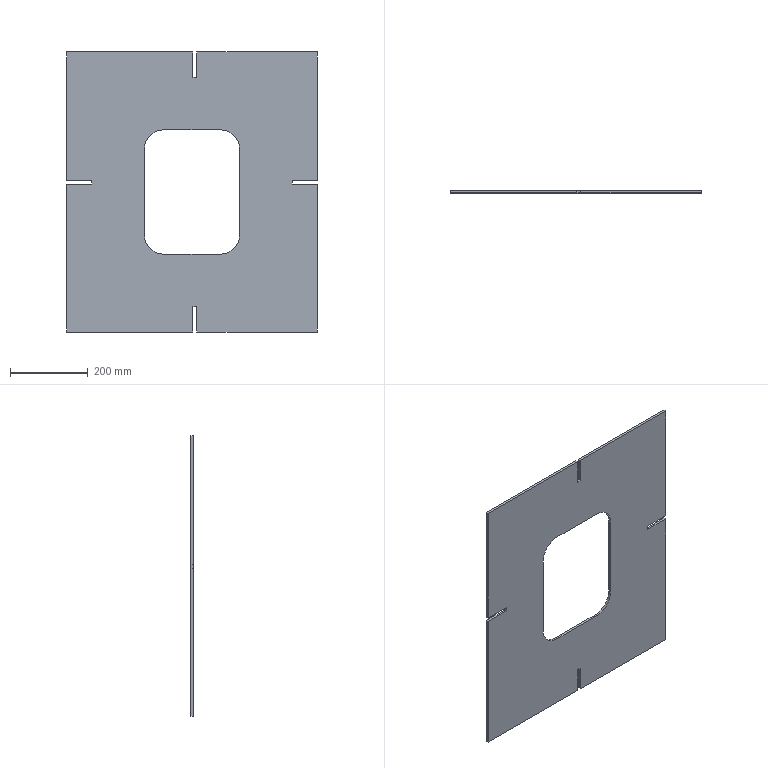Part | SolidWorks | features FlatPattern 1, SMBaseFlange 1, SheetMetal 1 | 1 solid | 30 faces | box 645 x 6 x 720 mm | volume 2313276 mm3 | plane 26 | cylinder 4 | commonest cylinder face diameters 100 x4
STEP:
#1=CARTESIAN_POINT('',(322.5,0.,360.));
#2=VERTEX_POINT('',#1);
#3=CARTESIAN_POINT('',(322.5,0.,30.));
#4=VERTEX_POINT('',#3);
#5=CARTESIAN_POINT('',(322.5,0.,30.));
#6=DIRECTION('',(0.,0.,-1.));
#7=VECTOR('',#6,1000.);
#8=LINE('',#5,#7);
#9=EDGE_CURVE('',#2,#4,#8,.T.);
#10=ORIENTED_EDGE('',*,*,#9,.F.);
#11=CARTESIAN_POINT('',(322.5,-6.,360.));
#12=VERTEX_POINT('',#11);
#13=CARTESIAN_POINT('',(322.5,-6.,360.));
#14=DIRECTION('',(0.,1.,0.));
#15=VECTOR('',#14,1000.);
#16=LINE('',#13,#15);
#17=EDGE_CURVE('',#12,#2,#16,.T.);
#18=ORIENTED_EDGE('',*,*,#17,.F.);
#19=CARTESIAN_POINT('',(322.5,-6.,30.));
#20=VERTEX_POINT('',#19);
#21=CARTESIAN_POINT('',(322.5,-6.,30.));
#22=DIRECTION('',(0.,0.,-1.));
#23=VECTOR('',#22,1000.);
#24=LINE('',#21,#23);
#25=EDGE_CURVE('',#12,#20,#24,.T.);
#26=ORIENTED_EDGE('',*,*,#25,.T.);
#27=CARTESIAN_POINT('',(322.5,-6.,30.));
#28=DIRECTION('',(0.,1.,0.));
#29=VECTOR('',#28,1000.);
#30=LINE('',#27,#29);
#31=EDGE_CURVE('',#20,#4,#30,.T.);
#32=ORIENTED_EDGE('',*,*,#31,.T.);
#33=EDGE_LOOP('',(#10,#18,#26,#32));
#34=FACE_OUTER_BOUND('',#33,.T.);
#35=CARTESIAN_POINT('',(322.5,-6.,30.));
#36=DIRECTION('',(1.,0.,0.));
#37=DIRECTION('',(0.,0.,-1.));
#38=AXIS2_PLACEMENT_3D('',#35,#36,#37);
#39=PLANE('',#38);
#40=ADVANCED_FACE('',(#34),#39,.T.);
#41=CARTESIAN_POINT('',(12.5,0.,360.));
#42=VERTEX_POINT('',#41);
#43=CARTESIAN_POINT('',(12.5,0.,360.));
#44=DIRECTION('',(1.,0.,0.));
#45=VECTOR('',#44,1000.);
#46=LINE('',#43,#45);
#47=EDGE_CURVE('',#42,#2,#46,.T.);
#48=ORIENTED_EDGE('',*,*,#47,.F.);
#49=CARTESIAN_POINT('',(12.5,-6.,360.));
#50=VERTEX_POINT('',#49);
#51=CARTESIAN_POINT('',(12.5,-6.,360.));
#52=DIRECTION('',(0.,1.,0.));
#53=VECTOR('',#52,1000.);
#54=LINE('',#51,#53);
#55=EDGE_CURVE('',#50,#42,#54,.T.);
#56=ORIENTED_EDGE('',*,*,#55,.F.);
#57=CARTESIAN_POINT('',(12.5,-6.,360.));
#58=DIRECTION('',(1.,0.,0.));
#59=VECTOR('',#58,1000.);
#60=LINE('',#57,#59);
#61=EDGE_CURVE('',#50,#12,#60,.T.);
#62=ORIENTED_EDGE('',*,*,#61,.T.);
#63=ORIENTED_EDGE('',*,*,#17,.T.);
#64=EDGE_LOOP('',(#48,#56,#62,#63));
#65=FACE_OUTER_BOUND('',#64,.T.);
#66=CARTESIAN_POINT('',(12.5,-6.,360.));
#67=DIRECTION('',(0.,0.,1.));
#68=DIRECTION('',(1.,0.,0.));
#69=AXIS2_PLACEMENT_3D('',#66,#67,#68);
#70=PLANE('',#69);
#71=ADVANCED_FACE('',(#65),#70,.T.);
#72=CARTESIAN_POINT('',(12.5,0.,295.));
#73=VERTEX_POINT('',#72);
#74=CARTESIAN_POINT('',(12.5,0.,295.));
#75=DIRECTION('',(0.,0.,1.));
#76=VECTOR('',#75,1000.);
#77=LINE('',#74,#76);
#78=EDGE_CURVE('',#73,#42,#77,.T.);
#79=ORIENTED_EDGE('',*,*,#78,.F.);
#80=CARTESIAN_POINT('',(12.5,-6.,295.));
#81=VERTEX_POINT('',#80);
#82=CARTESIAN_POINT('',(12.5,-6.,295.));
#83=DIRECTION('',(0.,1.,0.));
#84=VECTOR('',#83,1000.);
#85=LINE('',#82,#84);
#86=EDGE_CURVE('',#81,#73,#85,.T.);
#87=ORIENTED_EDGE('',*,*,#86,.F.);
#88=CARTESIAN_POINT('',(12.5,-6.,295.));
#89=DIRECTION('',(0.,0.,1.));
#90=VECTOR('',#89,1000.);
#91=LINE('',#88,#90);
#92=EDGE_CURVE('',#81,#50,#91,.T.);
#93=ORIENTED_EDGE('',*,*,#92,.T.);
#94=ORIENTED_EDGE('',*,*,#55,.T.);
#95=EDGE_LOOP('',(#79,#87,#93,#94));
#96=FACE_OUTER_BOUND('',#95,.T.);
#97=CARTESIAN_POINT('',(12.5,-6.,295.));
#98=DIRECTION('',(-1.,0.,0.));
#99=DIRECTION('',(0.,0.,1.));
#100=AXIS2_PLACEMENT_3D('',#97,#98,#99);
#101=PLANE('',#100);
#102=ADVANCED_FACE('',(#96),#101,.T.);
#103=CARTESIAN_POINT('',(2.5,0.,295.));
#104=VERTEX_POINT('',#103);
#105=CARTESIAN_POINT('',(2.5,0.,295.));
#106=DIRECTION('',(1.,0.,0.));
#107=VECTOR('',#106,1000.);
#108=LINE('',#105,#107);
#109=EDGE_CURVE('',#104,#73,#108,.T.);
#110=ORIENTED_EDGE('',*,*,#109,.F.);
#111=CARTESIAN_POINT('',(2.5,-6.,295.));
#112=VERTEX_POINT('',#111);
#113=CARTESIAN_POINT('',(2.5,-6.,295.));
#114=DIRECTION('',(0.,1.,0.));
#115=VECTOR('',#114,1000.);
#116=LINE('',#113,#115);
#117=EDGE_CURVE('',#112,#104,#116,.T.);
#118=ORIENTED_EDGE('',*,*,#117,.F.);
#119=CARTESIAN_POINT('',(2.5,-6.,295.));
#120=DIRECTION('',(1.,0.,0.));
#121=VECTOR('',#120,1000.);
#122=LINE('',#119,#121);
#123=EDGE_CURVE('',#112,#81,#122,.T.);
#124=ORIENTED_EDGE('',*,*,#123,.T.);
#125=ORIENTED_EDGE('',*,*,#86,.T.);
#126=EDGE_LOOP('',(#110,#118,#124,#125));
#127=FACE_OUTER_BOUND('',#126,.T.);
#128=CARTESIAN_POINT('',(2.5,-6.,295.));
#129=DIRECTION('',(0.,0.,1.));
#130=DIRECTION('',(1.,0.,0.));
#131=AXIS2_PLACEMENT_3D('',#128,#129,#130);
#132=PLANE('',#131);
#133=ADVANCED_FACE('',(#127),#132,.T.);
#134=CARTESIAN_POINT('',(2.5,0.,360.));
#135=VERTEX_POINT('',#134);
#136=CARTESIAN_POINT('',(2.5,0.,360.));
#137=DIRECTION('',(0.,0.,-1.));
#138=VECTOR('',#137,1000.);
#139=LINE('',#136,#138);
#140=EDGE_CURVE('',#135,#104,#139,.T.);
#141=ORIENTED_EDGE('',*,*,#140,.F.);
#142=CARTESIAN_POINT('',(2.5,-6.,360.));
#143=VERTEX_POINT('',#142);
#144=CARTESIAN_POINT('',(2.5,-6.,360.));
#145=DIRECTION('',(0.,1.,0.));
#146=VECTOR('',#145,1000.);
#147=LINE('',#144,#146);
#148=EDGE_CURVE('',#143,#135,#147,.T.);
#149=ORIENTED_EDGE('',*,*,#148,.F.);
#150=CARTESIAN_POINT('',(2.5,-6.,360.));
#151=DIRECTION('',(0.,0.,-1.));
#152=VECTOR('',#151,1000.);
#153=LINE('',#150,#152);
#154=EDGE_CURVE('',#143,#112,#153,.T.);
#155=ORIENTED_EDGE('',*,*,#154,.T.);
#156=ORIENTED_EDGE('',*,*,#117,.T.);
#157=EDGE_LOOP('',(#141,#149,#155,#156));
#158=FACE_OUTER_BOUND('',#157,.T.);
#159=CARTESIAN_POINT('',(2.5,-6.,360.));
#160=DIRECTION('',(1.,0.,0.));
#161=DIRECTION('',(0.,0.,-1.));
#162=AXIS2_PLACEMENT_3D('',#159,#160,#161);
#163=PLANE('',#162);
#164=ADVANCED_FACE('',(#158),#163,.T.);
#165=CARTESIAN_POINT('',(-322.5,0.,360.));
#166=VERTEX_POINT('',#165);
#167=CARTESIAN_POINT('',(-322.5,0.,360.));
#168=DIRECTION('',(1.,0.,0.));
#169=VECTOR('',#168,1000.);
#170=LINE('',#167,#169);
#171=EDGE_CURVE('',#166,#135,#170,.T.);
#172=ORIENTED_EDGE('',*,*,#171,.F.);
#173=CARTESIAN_POINT('',(-322.5,-6.,360.));
#174=VERTEX_POINT('',#173);
#175=CARTESIAN_POINT('',(-322.5,-6.,360.));
#176=DIRECTION('',(0.,1.,0.));
#177=VECTOR('',#176,1000.);
#178=LINE('',#175,#177);
#179=EDGE_CURVE('',#174,#166,#178,.T.);
#180=ORIENTED_EDGE('',*,*,#179,.F.);
#181=CARTESIAN_POINT('',(-322.5,-6.,360.));
#182=DIRECTION('',(1.,0.,0.));
#183=VECTOR('',#182,1000.);
#184=LINE('',#181,#183);
#185=EDGE_CURVE('',#174,#143,#184,.T.);
#186=ORIENTED_EDGE('',*,*,#185,.T.);
#187=ORIENTED_EDGE('',*,*,#148,.T.);
#188=EDGE_LOOP('',(#172,#180,#186,#187));
#189=FACE_OUTER_BOUND('',#188,.T.);
#190=CARTESIAN_POINT('',(-322.5,-6.,360.));
#191=DIRECTION('',(0.,0.,1.));
#192=DIRECTION('',(1.,0.,0.));
#193=AXIS2_PLACEMENT_3D('',#190,#191,#192);
#194=PLANE('',#193);
#195=ADVANCED_FACE('',(#189),#194,.T.);
#196=CARTESIAN_POINT('',(-322.5,0.,30.));
#197=VERTEX_POINT('',#196);
#198=CARTESIAN_POINT('',(-322.5,0.,30.));
#199=DIRECTION('',(0.,0.,1.));
#200=VECTOR('',#199,1000.);
#201=LINE('',#198,#200);
#202=EDGE_CURVE('',#197,#166,#201,.T.);
#203=ORIENTED_EDGE('',*,*,#202,.F.);
#204=CARTESIAN_POINT('',(-322.5,-6.,30.));
#205=VERTEX_POINT('',#204);
#206=CARTESIAN_POINT('',(-322.5,-6.,30.));
#207=DIRECTION('',(0.,1.,0.));
#208=VECTOR('',#207,1000.);
#209=LINE('',#206,#208);
#210=EDGE_CURVE('',#205,#197,#209,.T.);
#211=ORIENTED_EDGE('',*,*,#210,.F.);
#212=CARTESIAN_POINT('',(-322.5,-6.,30.));
#213=DIRECTION('',(0.,0.,1.));
#214=VECTOR('',#213,1000.);
#215=LINE('',#212,#214);
#216=EDGE_CURVE('',#205,#174,#215,.T.);
#217=ORIENTED_EDGE('',*,*,#216,.T.);
#218=ORIENTED_EDGE('',*,*,#179,.T.);
#219=EDGE_LOOP('',(#203,#211,#217,#218));
#220=FACE_OUTER_BOUND('',#219,.T.);
#221=CARTESIAN_POINT('',(-322.5,-6.,30.));
#222=DIRECTION('',(-1.,0.,0.));
#223=DIRECTION('',(0.,0.,1.));
#224=AXIS2_PLACEMENT_3D('',#221,#222,#223);
#225=PLANE('',#224);
#226=ADVANCED_FACE('',(#220),#225,.T.);
#227=CARTESIAN_POINT('',(-257.5,0.,30.));
#228=VERTEX_POINT('',#227);
#229=CARTESIAN_POINT('',(-257.5,0.,30.));
#230=DIRECTION('',(-1.,0.,0.));
#231=VECTOR('',#230,1000.);
#232=LINE('',#229,#231);
#233=EDGE_CURVE('',#228,#197,#232,.T.);
#234=ORIENTED_EDGE('',*,*,#233,.F.);
#235=CARTESIAN_POINT('',(-257.5,-6.,30.));
#236=VERTEX_POINT('',#235);
#237=CARTESIAN_POINT('',(-257.5,-6.,30.));
#238=DIRECTION('',(0.,1.,0.));
#239=VECTOR('',#238,1000.);
#240=LINE('',#237,#239);
#241=EDGE_CURVE('',#236,#228,#240,.T.);
#242=ORIENTED_EDGE('',*,*,#241,.F.);
#243=CARTESIAN_POINT('',(-257.5,-6.,30.));
#244=DIRECTION('',(-1.,0.,0.));
#245=VECTOR('',#244,1000.);
#246=LINE('',#243,#245);
#247=EDGE_CURVE('',#236,#205,#246,.T.);
#248=ORIENTED_EDGE('',*,*,#247,.T.);
#249=ORIENTED_EDGE('',*,*,#210,.T.);
#250=EDGE_LOOP('',(#234,#242,#248,#249));
#251=FACE_OUTER_BOUND('',#250,.T.);
#252=CARTESIAN_POINT('',(-257.5,-6.,30.));
#253=DIRECTION('',(0.,0.,-1.));
#254=DIRECTION('',(-1.,0.,0.));
#255=AXIS2_PLACEMENT_3D('',#252,#253,#254);
#256=PLANE('',#255);
#257=ADVANCED_FACE('',(#251),#256,.T.);
#258=CARTESIAN_POINT('',(-257.5,0.,20.));
#259=VERTEX_POINT('',#258);
#260=CARTESIAN_POINT('',(-257.5,0.,20.));
#261=DIRECTION('',(0.,0.,1.));
#262=VECTOR('',#261,1000.);
#263=LINE('',#260,#262);
#264=EDGE_CURVE('',#259,#228,#263,.T.);
#265=ORIENTED_EDGE('',*,*,#264,.F.);
#266=CARTESIAN_POINT('',(-257.5,-6.,20.));
#267=VERTEX_POINT('',#266);
#268=CARTESIAN_POINT('',(-257.5,-6.,20.));
#269=DIRECTION('',(0.,1.,0.));
#270=VECTOR('',#269,1000.);
#271=LINE('',#268,#270);
#272=EDGE_CURVE('',#267,#259,#271,.T.);
#273=ORIENTED_EDGE('',*,*,#272,.F.);
#274=CARTESIAN_POINT('',(-257.5,-6.,20.));
#275=DIRECTION('',(0.,0.,1.));
#276=VECTOR('',#275,1000.);
#277=LINE('',#274,#276);
#278=EDGE_CURVE('',#267,#236,#277,.T.);
#279=ORIENTED_EDGE('',*,*,#278,.T.);
#280=ORIENTED_EDGE('',*,*,#241,.T.);
#281=EDGE_LOOP('',(#265,#273,#279,#280));
#282=FACE_OUTER_BOUND('',#281,.T.);
#283=CARTESIAN_POINT('',(-257.5,-6.,20.));
#284=DIRECTION('',(-1.,0.,0.));
#285=DIRECTION('',(0.,0.,1.));
#286=AXIS2_PLACEMENT_3D('',#283,#284,#285);
#287=PLANE('',#286);
#288=ADVANCED_FACE('',(#282),#287,.T.);
#289=CARTESIAN_POINT('',(-322.5,0.,20.));
#290=VERTEX_POINT('',#289);
#291=CARTESIAN_POINT('',(-322.5,0.,20.));
#292=DIRECTION('',(1.,0.,0.));
#293=VECTOR('',#292,1000.);
#294=LINE('',#291,#293);
#295=EDGE_CURVE('',#290,#259,#294,.T.);
#296=ORIENTED_EDGE('',*,*,#295,.F.);
#297=CARTESIAN_POINT('',(-322.5,-6.,20.));
#298=VERTEX_POINT('',#297);
#299=CARTESIAN_POINT('',(-322.5,-6.,20.));
#300=DIRECTION('',(0.,1.,0.));
#301=VECTOR('',#300,1000.);
#302=LINE('',#299,#301);
#303=EDGE_CURVE('',#298,#290,#302,.T.);
#304=ORIENTED_EDGE('',*,*,#303,.F.);
#305=CARTESIAN_POINT('',(-322.5,-6.,20.));
#306=DIRECTION('',(1.,0.,0.));
#307=VECTOR('',#306,1000.);
#308=LINE('',#305,#307);
#309=EDGE_CURVE('',#298,#267,#308,.T.);
#310=ORIENTED_EDGE('',*,*,#309,.T.);
#311=ORIENTED_EDGE('',*,*,#272,.T.);
#312=EDGE_LOOP('',(#296,#304,#310,#311));
#313=FACE_OUTER_BOUND('',#312,.T.);
#314=CARTESIAN_POINT('',(-322.5,-6.,20.));
#315=DIRECTION('',(0.,0.,1.));
#316=DIRECTION('',(1.,0.,0.));
#317=AXIS2_PLACEMENT_3D('',#314,#315,#316);
#318=PLANE('',#317);
#319=ADVANCED_FACE('',(#313),#318,.T.);
#320=CARTESIAN_POINT('',(-322.5,0.,-360.));
#321=VERTEX_POINT('',#320);
#322=CARTESIAN_POINT('',(-322.5,0.,-360.));
#323=DIRECTION('',(0.,0.,1.));
#324=VECTOR('',#323,1000.);
#325=LINE('',#322,#324);
#326=EDGE_CURVE('',#321,#290,#325,.T.);
#327=ORIENTED_EDGE('',*,*,#326,.F.);
#328=CARTESIAN_POINT('',(-322.5,-6.,-360.));
#329=VERTEX_POINT('',#328);
#330=CARTESIAN_POINT('',(-322.5,-6.,-360.));
#331=DIRECTION('',(0.,1.,0.));
#332=VECTOR('',#331,1000.);
#333=LINE('',#330,#332);
#334=EDGE_CURVE('',#329,#321,#333,.T.);
#335=ORIENTED_EDGE('',*,*,#334,.F.);
#336=CARTESIAN_POINT('',(-322.5,-6.,-360.));
#337=DIRECTION('',(0.,0.,1.));
#338=VECTOR('',#337,1000.);
#339=LINE('',#336,#338);
#340=EDGE_CURVE('',#329,#298,#339,.T.);
#341=ORIENTED_EDGE('',*,*,#340,.T.);
#342=ORIENTED_EDGE('',*,*,#303,.T.);
#343=EDGE_LOOP('',(#327,#335,#341,#342));
#344=FACE_OUTER_BOUND('',#343,.T.);
#345=CARTESIAN_POINT('',(-322.5,-6.,-360.));
#346=DIRECTION('',(-1.,0.,0.));
#347=DIRECTION('',(0.,0.,1.));
#348=AXIS2_PLACEMENT_3D('',#345,#346,#347);
#349=PLANE('',#348);
#350=ADVANCED_FACE('',(#344),#349,.T.);
#351=CARTESIAN_POINT('',(2.5,0.,-360.));
#352=VERTEX_POINT('',#351);
#353=CARTESIAN_POINT('',(-322.5,0.,-360.));
#354=DIRECTION('',(-1.,0.,0.));
#355=VECTOR('',#354,1000.);
#356=LINE('',#353,#355);
#357=EDGE_CURVE('',#352,#321,#356,.T.);
#358=ORIENTED_EDGE('',*,*,#357,.F.);
#359=CARTESIAN_POINT('',(2.5,-6.,-360.));
#360=VERTEX_POINT('',#359);
#361=CARTESIAN_POINT('',(2.5,-6.,-360.));
#362=DIRECTION('',(0.,1.,0.));
#363=VECTOR('',#362,1000.);
#364=LINE('',#361,#363);
#365=EDGE_CURVE('',#360,#352,#364,.T.);
#366=ORIENTED_EDGE('',*,*,#365,.F.);
#367=CARTESIAN_POINT('',(-322.5,-6.,-360.));
#368=DIRECTION('',(-1.,0.,0.));
#369=VECTOR('',#368,1000.);
#370=LINE('',#367,#369);
#371=EDGE_CURVE('',#360,#329,#370,.T.);
#372=ORIENTED_EDGE('',*,*,#371,.T.);
#373=ORIENTED_EDGE('',*,*,#334,.T.);
#374=EDGE_LOOP('',(#358,#366,#372,#373));
#375=FACE_OUTER_BOUND('',#374,.T.);
#376=CARTESIAN_POINT('',(-322.5,-6.,-360.));
#377=DIRECTION('',(0.,0.,-1.));
#378=DIRECTION('',(-1.,0.,0.));
#379=AXIS2_PLACEMENT_3D('',#376,#377,#378);
#380=PLANE('',#379);
#381=ADVANCED_FACE('',(#375),#380,.T.);
#382=CARTESIAN_POINT('',(2.5,0.,-295.));
#383=VERTEX_POINT('',#382);
#384=CARTESIAN_POINT('',(2.5,0.,-360.));
#385=DIRECTION('',(0.,0.,-1.));
#386=VECTOR('',#385,1000.);
#387=LINE('',#384,#386);
#388=EDGE_CURVE('',#383,#352,#387,.T.);
#389=ORIENTED_EDGE('',*,*,#388,.F.);
#390=CARTESIAN_POINT('',(2.5,-6.,-295.));
#391=VERTEX_POINT('',#390);
#392=CARTESIAN_POINT('',(2.5,-6.,-295.));
#393=DIRECTION('',(0.,1.,0.));
#394=VECTOR('',#393,1000.);
#395=LINE('',#392,#394);
#396=EDGE_CURVE('',#391,#383,#395,.T.);
#397=ORIENTED_EDGE('',*,*,#396,.F.);
#398=CARTESIAN_POINT('',(2.5,-6.,-360.));
#399=DIRECTION('',(0.,0.,-1.));
#400=VECTOR('',#399,1000.);
#401=LINE('',#398,#400);
#402=EDGE_CURVE('',#391,#360,#401,.T.);
#403=ORIENTED_EDGE('',*,*,#402,.T.);
#404=ORIENTED_EDGE('',*,*,#365,.T.);
#405=EDGE_LOOP('',(#389,#397,#403,#404));
#406=FACE_OUTER_BOUND('',#405,.T.);
#407=CARTESIAN_POINT('',(2.5,-6.,-360.));
#408=DIRECTION('',(1.,0.,0.));
#409=DIRECTION('',(0.,0.,-1.));
#410=AXIS2_PLACEMENT_3D('',#407,#408,#409);
#411=PLANE('',#410);
#412=ADVANCED_FACE('',(#406),#411,.T.);
#413=CARTESIAN_POINT('',(12.5,0.,-295.));
#414=VERTEX_POINT('',#413);
#415=CARTESIAN_POINT('',(2.5,0.,-295.));
#416=DIRECTION('',(-1.,0.,0.));
#417=VECTOR('',#416,1000.);
#418=LINE('',#415,#417);
#419=EDGE_CURVE('',#414,#383,#418,.T.);
#420=ORIENTED_EDGE('',*,*,#419,.F.);
#421=CARTESIAN_POINT('',(12.5,-6.,-295.));
#422=VERTEX_POINT('',#421);
#423=CARTESIAN_POINT('',(12.5,-6.,-295.));
#424=DIRECTION('',(0.,1.,0.));
#425=VECTOR('',#424,1000.);
#426=LINE('',#423,#425);
#427=EDGE_CURVE('',#422,#414,#426,.T.);
#428=ORIENTED_EDGE('',*,*,#427,.F.);
#429=CARTESIAN_POINT('',(2.5,-6.,-295.));
#430=DIRECTION('',(-1.,0.,0.));
#431=VECTOR('',#430,1000.);
#432=LINE('',#429,#431);
#433=EDGE_CURVE('',#422,#391,#432,.T.);
#434=ORIENTED_EDGE('',*,*,#433,.T.);
#435=ORIENTED_EDGE('',*,*,#396,.T.);
#436=EDGE_LOOP('',(#420,#428,#434,#435));
#437=FACE_OUTER_BOUND('',#436,.T.);
#438=CARTESIAN_POINT('',(2.5,-6.,-295.));
#439=DIRECTION('',(0.,0.,-1.));
#440=DIRECTION('',(-1.,0.,0.));
#441=AXIS2_PLACEMENT_3D('',#438,#439,#440);
#442=PLANE('',#441);
#443=ADVANCED_FACE('',(#437),#442,.T.);
#444=CARTESIAN_POINT('',(12.5,0.,-360.));
#445=VERTEX_POINT('',#444);
#446=CARTESIAN_POINT('',(12.5,0.,-295.));
#447=DIRECTION('',(0.,0.,1.));
#448=VECTOR('',#447,1000.);
#449=LINE('',#446,#448);
#450=EDGE_CURVE('',#445,#414,#449,.T.);
#451=ORIENTED_EDGE('',*,*,#450,.F.);
#452=CARTESIAN_POINT('',(12.5,-6.,-360.));
#453=VERTEX_POINT('',#452);
#454=CARTESIAN_POINT('',(12.5,-6.,-360.));
#455=DIRECTION('',(0.,1.,0.));
#456=VECTOR('',#455,1000.);
#457=LINE('',#454,#456);
#458=EDGE_CURVE('',#453,#445,#457,.T.);
#459=ORIENTED_EDGE('',*,*,#458,.F.);
#460=CARTESIAN_POINT('',(12.5,-6.,-295.));
#461=DIRECTION('',(0.,0.,1.));
#462=VECTOR('',#461,1000.);
#463=LINE('',#460,#462);
#464=EDGE_CURVE('',#453,#422,#463,.T.);
#465=ORIENTED_EDGE('',*,*,#464,.T.);
#466=ORIENTED_EDGE('',*,*,#427,.T.);
#467=EDGE_LOOP('',(#451,#459,#465,#466));
#468=FACE_OUTER_BOUND('',#467,.T.);
#469=CARTESIAN_POINT('',(12.5,-6.,-295.));
#470=DIRECTION('',(-1.,0.,0.));
#471=DIRECTION('',(0.,0.,1.));
#472=AXIS2_PLACEMENT_3D('',#469,#470,#471);
#473=PLANE('',#472);
#474=ADVANCED_FACE('',(#468),#473,.T.);
#475=CARTESIAN_POINT('',(322.5,0.,-360.));
#476=VERTEX_POINT('',#475);
#477=CARTESIAN_POINT('',(12.5,0.,-360.));
#478=DIRECTION('',(-1.,0.,0.));
#479=VECTOR('',#478,1000.);
#480=LINE('',#477,#479);
#481=EDGE_CURVE('',#476,#445,#480,.T.);
#482=ORIENTED_EDGE('',*,*,#481,.F.);
#483=CARTESIAN_POINT('',(322.5,-6.,-360.));
#484=VERTEX_POINT('',#483);
#485=CARTESIAN_POINT('',(322.5,-6.,-360.));
#486=DIRECTION('',(0.,1.,0.));
#487=VECTOR('',#486,1000.);
#488=LINE('',#485,#487);
#489=EDGE_CURVE('',#484,#476,#488,.T.);
#490=ORIENTED_EDGE('',*,*,#489,.F.);
#491=CARTESIAN_POINT('',(12.5,-6.,-360.));
#492=DIRECTION('',(-1.,0.,0.));
#493=VECTOR('',#492,1000.);
#494=LINE('',#491,#493);
#495=EDGE_CURVE('',#484,#453,#494,.T.);
#496=ORIENTED_EDGE('',*,*,#495,.T.);
#497=ORIENTED_EDGE('',*,*,#458,.T.);
#498=EDGE_LOOP('',(#482,#490,#496,#497));
#499=FACE_OUTER_BOUND('',#498,.T.);
#500=CARTESIAN_POINT('',(12.5,-6.,-360.));
#501=DIRECTION('',(0.,0.,-1.));
#502=DIRECTION('',(-1.,0.,0.));
#503=AXIS2_PLACEMENT_3D('',#500,#501,#502);
#504=PLANE('',#503);
#505=ADVANCED_FACE('',(#499),#504,.T.);
#506=CARTESIAN_POINT('',(322.5,0.,20.));
#507=VERTEX_POINT('',#506);
#508=CARTESIAN_POINT('',(322.5,0.,-360.));
#509=DIRECTION('',(0.,0.,-1.));
#510=VECTOR('',#509,1000.);
#511=LINE('',#508,#510);
#512=EDGE_CURVE('',#507,#476,#511,.T.);
#513=ORIENTED_EDGE('',*,*,#512,.F.);
#514=CARTESIAN_POINT('',(322.5,-6.,20.));
#515=VERTEX_POINT('',#514);
#516=CARTESIAN_POINT('',(322.5,-6.,20.));
#517=DIRECTION('',(0.,1.,0.));
#518=VECTOR('',#517,1000.);
#519=LINE('',#516,#518);
#520=EDGE_CURVE('',#515,#507,#519,.T.);
#521=ORIENTED_EDGE('',*,*,#520,.F.);
#522=CARTESIAN_POINT('',(322.5,-6.,-360.));
#523=DIRECTION('',(0.,0.,-1.));
#524=VECTOR('',#523,1000.);
#525=LINE('',#522,#524);
#526=EDGE_CURVE('',#515,#484,#525,.T.);
#527=ORIENTED_EDGE('',*,*,#526,.T.);
#528=ORIENTED_EDGE('',*,*,#489,.T.);
#529=EDGE_LOOP('',(#513,#521,#527,#528));
#530=FACE_OUTER_BOUND('',#529,.T.);
#531=CARTESIAN_POINT('',(322.5,-6.,-360.));
#532=DIRECTION('',(1.,0.,0.));
#533=DIRECTION('',(0.,0.,-1.));
#534=AXIS2_PLACEMENT_3D('',#531,#532,#533);
#535=PLANE('',#534);
#536=ADVANCED_FACE('',(#530),#535,.T.);
#537=CARTESIAN_POINT('',(257.5,0.,20.));
#538=VERTEX_POINT('',#537);
#539=CARTESIAN_POINT('',(322.5,0.,20.));
#540=DIRECTION('',(1.,0.,0.));
#541=VECTOR('',#540,1000.);
#542=LINE('',#539,#541);
#543=EDGE_CURVE('',#538,#507,#542,.T.);
#544=ORIENTED_EDGE('',*,*,#543,.F.);
#545=CARTESIAN_POINT('',(257.5,-6.,20.));
#546=VERTEX_POINT('',#545);
#547=CARTESIAN_POINT('',(257.5,-6.,20.));
#548=DIRECTION('',(0.,1.,0.));
#549=VECTOR('',#548,1000.);
#550=LINE('',#547,#549);
#551=EDGE_CURVE('',#546,#538,#550,.T.);
#552=ORIENTED_EDGE('',*,*,#551,.F.);
#553=CARTESIAN_POINT('',(322.5,-6.,20.));
#554=DIRECTION('',(1.,0.,0.));
#555=VECTOR('',#554,1000.);
#556=LINE('',#553,#555);
#557=EDGE_CURVE('',#546,#515,#556,.T.);
#558=ORIENTED_EDGE('',*,*,#557,.T.);
#559=ORIENTED_EDGE('',*,*,#520,.T.);
#560=EDGE_LOOP('',(#544,#552,#558,#559));
#561=FACE_OUTER_BOUND('',#560,.T.);
#562=CARTESIAN_POINT('',(322.5,-6.,20.));
#563=DIRECTION('',(0.,0.,1.));
#564=DIRECTION('',(1.,0.,0.));
#565=AXIS2_PLACEMENT_3D('',#562,#563,#564);
#566=PLANE('',#565);
#567=ADVANCED_FACE('',(#561),#566,.T.);
#568=CARTESIAN_POINT('',(257.5,0.,30.));
#569=VERTEX_POINT('',#568);
#570=CARTESIAN_POINT('',(257.5,0.,20.));
#571=DIRECTION('',(0.,0.,-1.));
#572=VECTOR('',#571,1000.);
#573=LINE('',#570,#572);
#574=EDGE_CURVE('',#569,#538,#573,.T.);
#575=ORIENTED_EDGE('',*,*,#574,.F.);
#576=CARTESIAN_POINT('',(257.5,-6.,30.));
#577=VERTEX_POINT('',#576);
#578=CARTESIAN_POINT('',(257.5,-6.,30.));
#579=DIRECTION('',(0.,1.,0.));
#580=VECTOR('',#579,1000.);
#581=LINE('',#578,#580);
#582=EDGE_CURVE('',#577,#569,#581,.T.);
#583=ORIENTED_EDGE('',*,*,#582,.F.);
#584=CARTESIAN_POINT('',(257.5,-6.,20.));
#585=DIRECTION('',(0.,0.,-1.));
#586=VECTOR('',#585,1000.);
#587=LINE('',#584,#586);
#588=EDGE_CURVE('',#577,#546,#587,.T.);
#589=ORIENTED_EDGE('',*,*,#588,.T.);
#590=ORIENTED_EDGE('',*,*,#551,.T.);
#591=EDGE_LOOP('',(#575,#583,#589,#590));
#592=FACE_OUTER_BOUND('',#591,.T.);
#593=CARTESIAN_POINT('',(257.5,-6.,20.));
#594=DIRECTION('',(1.,0.,0.));
#595=DIRECTION('',(0.,0.,-1.));
#596=AXIS2_PLACEMENT_3D('',#593,#594,#595);
#597=PLANE('',#596);
#598=ADVANCED_FACE('',(#592),#597,.T.);
#599=CARTESIAN_POINT('',(257.5,0.,30.));
#600=DIRECTION('',(-1.,0.,0.));
#601=VECTOR('',#600,1000.);
#602=LINE('',#599,#601);
#603=EDGE_CURVE('',#4,#569,#602,.T.);
#604=ORIENTED_EDGE('',*,*,#603,.F.);
#605=ORIENTED_EDGE('',*,*,#31,.F.);
#606=CARTESIAN_POINT('',(257.5,-6.,30.));
#607=DIRECTION('',(-1.,0.,0.));
#608=VECTOR('',#607,1000.);
#609=LINE('',#606,#608);
#610=EDGE_CURVE('',#20,#577,#609,.T.);
#611=ORIENTED_EDGE('',*,*,#610,.T.);
#612=ORIENTED_EDGE('',*,*,#582,.T.);
#613=EDGE_LOOP('',(#604,#605,#611,#612));
#614=FACE_OUTER_BOUND('',#613,.T.);
#615=CARTESIAN_POINT('',(257.5,-6.,30.));
#616=DIRECTION('',(0.,0.,-1.));
#617=DIRECTION('',(-1.,0.,0.));
#618=AXIS2_PLACEMENT_3D('',#615,#616,#617);
#619=PLANE('',#618);
#620=ADVANCED_FACE('',(#614),#619,.T.);
#621=CARTESIAN_POINT('',(-72.5,-6.,160.));
#622=VERTEX_POINT('',#621);
#623=CARTESIAN_POINT('',(72.5,-6.,160.));
#624=VERTEX_POINT('',#623);
#625=CARTESIAN_POINT('',(-72.5,-6.,160.));
#626=DIRECTION('',(1.,0.,0.));
#627=VECTOR('',#626,1000.);
#628=LINE('',#625,#627);
#629=EDGE_CURVE('',#622,#624,#628,.T.);
#630=ORIENTED_EDGE('',*,*,#629,.T.);
#631=CARTESIAN_POINT('',(122.5,-6.,110.));
#632=VERTEX_POINT('',#631);
#633=CARTESIAN_POINT('',(72.5,-6.,110.));
#634=DIRECTION('',(0.,1.,0.));
#635=DIRECTION('',(0.,0.,1.));
#636=AXIS2_PLACEMENT_3D('',#633,#634,#635);
#637=CIRCLE('',#636,50.);
#638=EDGE_CURVE('',#624,#632,#637,.T.);
#639=ORIENTED_EDGE('',*,*,#638,.T.);
#640=CARTESIAN_POINT('',(122.5,-6.,-110.));
#641=VERTEX_POINT('',#640);
#642=CARTESIAN_POINT('',(122.5,-6.,110.));
#643=DIRECTION('',(0.,0.,-1.));
#644=VECTOR('',#643,1000.);
#645=LINE('',#642,#644);
#646=EDGE_CURVE('',#632,#641,#645,.T.);
#647=ORIENTED_EDGE('',*,*,#646,.T.);
#648=CARTESIAN_POINT('',(72.5,-6.,-160.));
#649=VERTEX_POINT('',#648);
#650=CARTESIAN_POINT('',(72.5,-6.,-110.));
#651=DIRECTION('',(0.,1.,0.));
#652=DIRECTION('',(0.,0.,-1.));
#653=AXIS2_PLACEMENT_3D('',#650,#651,#652);
#654=CIRCLE('',#653,50.);
#655=EDGE_CURVE('',#641,#649,#654,.T.);
#656=ORIENTED_EDGE('',*,*,#655,.T.);
#657=CARTESIAN_POINT('',(-72.5,-6.,-160.));
#658=VERTEX_POINT('',#657);
#659=CARTESIAN_POINT('',(-72.5,-6.,-160.));
#660=DIRECTION('',(-1.,0.,0.));
#661=VECTOR('',#660,1000.);
#662=LINE('',#659,#661);
#663=EDGE_CURVE('',#649,#658,#662,.T.);
#664=ORIENTED_EDGE('',*,*,#663,.T.);
#665=CARTESIAN_POINT('',(-122.5,-6.,-110.));
#666=VERTEX_POINT('',#665);
#667=CARTESIAN_POINT('',(-72.5,-6.,-110.));
#668=DIRECTION('',(0.,1.,0.));
#669=DIRECTION('',(0.,0.,-1.));
#670=AXIS2_PLACEMENT_3D('',#667,#668,#669);
#671=CIRCLE('',#670,50.);
#672=EDGE_CURVE('',#658,#666,#671,.T.);
#673=ORIENTED_EDGE('',*,*,#672,.T.);
#674=CARTESIAN_POINT('',(-122.5,-6.,110.));
#675=VERTEX_POINT('',#674);
#676=CARTESIAN_POINT('',(-122.5,-6.,110.));
#677=DIRECTION('',(0.,0.,1.));
#678=VECTOR('',#677,1000.);
#679=LINE('',#676,#678);
#680=EDGE_CURVE('',#666,#675,#679,.T.);
#681=ORIENTED_EDGE('',*,*,#680,.T.);
#682=CARTESIAN_POINT('',(-72.5,-6.,110.));
#683=DIRECTION('',(0.,1.,0.));
#684=DIRECTION('',(0.,0.,-1.));
#685=AXIS2_PLACEMENT_3D('',#682,#683,#684);
#686=CIRCLE('',#685,50.);
#687=EDGE_CURVE('',#675,#622,#686,.T.);
#688=ORIENTED_EDGE('',*,*,#687,.T.);
#689=EDGE_LOOP('',(#630,#639,#647,#656,#664,#673,#681,#688));
#690=FACE_BOUND('',#689,.T.);
#691=ORIENTED_EDGE('',*,*,#25,.F.);
#692=ORIENTED_EDGE('',*,*,#61,.F.);
#693=ORIENTED_EDGE('',*,*,#92,.F.);
#694=ORIENTED_EDGE('',*,*,#123,.F.);
#695=ORIENTED_EDGE('',*,*,#154,.F.);
#696=ORIENTED_EDGE('',*,*,#185,.F.);
#697=ORIENTED_EDGE('',*,*,#216,.F.);
#698=ORIENTED_EDGE('',*,*,#247,.F.);
#699=ORIENTED_EDGE('',*,*,#278,.F.);
#700=ORIENTED_EDGE('',*,*,#309,.F.);
#701=ORIENTED_EDGE('',*,*,#340,.F.);
#702=ORIENTED_EDGE('',*,*,#371,.F.);
#703=ORIENTED_EDGE('',*,*,#402,.F.);
#704=ORIENTED_EDGE('',*,*,#433,.F.);
#705=ORIENTED_EDGE('',*,*,#464,.F.);
#706=ORIENTED_EDGE('',*,*,#495,.F.);
#707=ORIENTED_EDGE('',*,*,#526,.F.);
#708=ORIENTED_EDGE('',*,*,#557,.F.);
#709=ORIENTED_EDGE('',*,*,#588,.F.);
#710=ORIENTED_EDGE('',*,*,#610,.F.);
#711=EDGE_LOOP('',(#691,#692,#693,#694,#695,#696,#697,#698,#699,#700,#701,#702,#703,#704,#705,#706,#707,#708,#709,#710));
#712=FACE_OUTER_BOUND('',#711,.T.);
#713=CARTESIAN_POINT('',(0.,-6.,0.));
#714=DIRECTION('',(0.,1.,0.));
#715=DIRECTION('',(0.,0.,1.));
#716=AXIS2_PLACEMENT_3D('',#713,#714,#715);
#717=PLANE('',#716);
#718=ADVANCED_FACE('',(#690,#712),#717,.F.);
#719=CARTESIAN_POINT('',(72.5,0.,160.));
#720=VERTEX_POINT('',#719);
#721=CARTESIAN_POINT('',(122.5,0.,110.));
#722=VERTEX_POINT('',#721);
#723=CARTESIAN_POINT('',(72.5,0.,110.));
#724=DIRECTION('',(0.,1.,0.));
#725=DIRECTION('',(0.,0.,1.));
#726=AXIS2_PLACEMENT_3D('',#723,#724,#725);
#727=CIRCLE('',#726,50.);
#728=EDGE_CURVE('',#720,#722,#727,.T.);
#729=ORIENTED_EDGE('',*,*,#728,.F.);
#730=CARTESIAN_POINT('',(-72.5,0.,160.));
#731=VERTEX_POINT('',#730);
#732=CARTESIAN_POINT('',(-72.5,0.,160.));
#733=DIRECTION('',(1.,0.,0.));
#734=VECTOR('',#733,1000.);
#735=LINE('',#732,#734);
#736=EDGE_CURVE('',#731,#720,#735,.T.);
#737=ORIENTED_EDGE('',*,*,#736,.F.);
#738=CARTESIAN_POINT('',(-122.5,0.,110.));
#739=VERTEX_POINT('',#738);
#740=CARTESIAN_POINT('',(-72.5,0.,110.));
#741=DIRECTION('',(0.,1.,0.));
#742=DIRECTION('',(0.,0.,-1.));
#743=AXIS2_PLACEMENT_3D('',#740,#741,#742);
#744=CIRCLE('',#743,50.);
#745=EDGE_CURVE('',#739,#731,#744,.T.);
#746=ORIENTED_EDGE('',*,*,#745,.F.);
#747=CARTESIAN_POINT('',(-122.5,0.,-110.));
#748=VERTEX_POINT('',#747);
#749=CARTESIAN_POINT('',(-122.5,0.,110.));
#750=DIRECTION('',(0.,0.,1.));
#751=VECTOR('',#750,1000.);
#752=LINE('',#749,#751);
#753=EDGE_CURVE('',#748,#739,#752,.T.);
#754=ORIENTED_EDGE('',*,*,#753,.F.);
#755=CARTESIAN_POINT('',(-72.5,0.,-160.));
#756=VERTEX_POINT('',#755);
#757=CARTESIAN_POINT('',(-72.5,0.,-110.));
#758=DIRECTION('',(0.,1.,0.));
#759=DIRECTION('',(0.,0.,-1.));
#760=AXIS2_PLACEMENT_3D('',#757,#758,#759);
#761=CIRCLE('',#760,50.);
#762=EDGE_CURVE('',#756,#748,#761,.T.);
#763=ORIENTED_EDGE('',*,*,#762,.F.);
#764=CARTESIAN_POINT('',(72.5,0.,-160.));
#765=VERTEX_POINT('',#764);
#766=CARTESIAN_POINT('',(-72.5,0.,-160.));
#767=DIRECTION('',(-1.,0.,0.));
#768=VECTOR('',#767,1000.);
#769=LINE('',#766,#768);
#770=EDGE_CURVE('',#765,#756,#769,.T.);
#771=ORIENTED_EDGE('',*,*,#770,.F.);
#772=CARTESIAN_POINT('',(122.5,0.,-110.));
#773=VERTEX_POINT('',#772);
#774=CARTESIAN_POINT('',(72.5,0.,-110.));
#775=DIRECTION('',(0.,1.,0.));
#776=DIRECTION('',(0.,0.,-1.));
#777=AXIS2_PLACEMENT_3D('',#774,#775,#776);
#778=CIRCLE('',#777,50.);
#779=EDGE_CURVE('',#773,#765,#778,.T.);
#780=ORIENTED_EDGE('',*,*,#779,.F.);
#781=CARTESIAN_POINT('',(122.5,0.,110.));
#782=DIRECTION('',(0.,0.,-1.));
#783=VECTOR('',#782,1000.);
#784=LINE('',#781,#783);
#785=EDGE_CURVE('',#722,#773,#784,.T.);
#786=ORIENTED_EDGE('',*,*,#785,.F.);
#787=EDGE_LOOP('',(#729,#737,#746,#754,#763,#771,#780,#786));
#788=FACE_BOUND('',#787,.T.);
#789=ORIENTED_EDGE('',*,*,#9,.T.);
#790=ORIENTED_EDGE('',*,*,#603,.T.);
#791=ORIENTED_EDGE('',*,*,#574,.T.);
#792=ORIENTED_EDGE('',*,*,#543,.T.);
#793=ORIENTED_EDGE('',*,*,#512,.T.);
#794=ORIENTED_EDGE('',*,*,#481,.T.);
#795=ORIENTED_EDGE('',*,*,#450,.T.);
#796=ORIENTED_EDGE('',*,*,#419,.T.);
#797=ORIENTED_EDGE('',*,*,#388,.T.);
#798=ORIENTED_EDGE('',*,*,#357,.T.);
#799=ORIENTED_EDGE('',*,*,#326,.T.);
#800=ORIENTED_EDGE('',*,*,#295,.T.);
#801=ORIENTED_EDGE('',*,*,#264,.T.);
#802=ORIENTED_EDGE('',*,*,#233,.T.);
#803=ORIENTED_EDGE('',*,*,#202,.T.);
#804=ORIENTED_EDGE('',*,*,#171,.T.);
#805=ORIENTED_EDGE('',*,*,#140,.T.);
#806=ORIENTED_EDGE('',*,*,#109,.T.);
#807=ORIENTED_EDGE('',*,*,#78,.T.);
#808=ORIENTED_EDGE('',*,*,#47,.T.);
#809=EDGE_LOOP('',(#789,#790,#791,#792,#793,#794,#795,#796,#797,#798,#799,#800,#801,#802,#803,#804,#805,#806,#807,#808));
#810=FACE_OUTER_BOUND('',#809,.T.);
#811=CARTESIAN_POINT('',(0.,0.,0.));
#812=DIRECTION('',(0.,1.,0.));
#813=DIRECTION('',(0.,0.,1.));
#814=AXIS2_PLACEMENT_3D('',#811,#812,#813);
#815=PLANE('',#814);
#816=ADVANCED_FACE('',(#788,#810),#815,.T.);
#817=ORIENTED_EDGE('',*,*,#728,.T.);
#818=CARTESIAN_POINT('',(122.5,-6.,110.));
#819=DIRECTION('',(0.,1.,0.));
#820=VECTOR('',#819,1000.);
#821=LINE('',#818,#820);
#822=EDGE_CURVE('',#632,#722,#821,.T.);
#823=ORIENTED_EDGE('',*,*,#822,.F.);
#824=ORIENTED_EDGE('',*,*,#638,.F.);
#825=CARTESIAN_POINT('',(72.5,-6.,160.));
#826=DIRECTION('',(0.,1.,0.));
#827=VECTOR('',#826,1000.);
#828=LINE('',#825,#827);
#829=EDGE_CURVE('',#624,#720,#828,.T.);
#830=ORIENTED_EDGE('',*,*,#829,.T.);
#831=EDGE_LOOP('',(#817,#823,#824,#830));
#832=FACE_OUTER_BOUND('',#831,.T.);
#833=CARTESIAN_POINT('',(72.5,-6.,110.));
#834=DIRECTION('',(0.,1.,0.));
#835=DIRECTION('',(0.,0.,1.));
#836=AXIS2_PLACEMENT_3D('',#833,#834,#835);
#837=CYLINDRICAL_SURFACE('',#836,50.);
#838=ADVANCED_FACE('',(#832),#837,.F.);
#839=ORIENTED_EDGE('',*,*,#736,.T.);
#840=ORIENTED_EDGE('',*,*,#829,.F.);
#841=ORIENTED_EDGE('',*,*,#629,.F.);
#842=CARTESIAN_POINT('',(-72.5,-6.,160.));
#843=DIRECTION('',(0.,1.,0.));
#844=VECTOR('',#843,1000.);
#845=LINE('',#842,#844);
#846=EDGE_CURVE('',#622,#731,#845,.T.);
#847=ORIENTED_EDGE('',*,*,#846,.T.);
#848=EDGE_LOOP('',(#839,#840,#841,#847));
#849=FACE_OUTER_BOUND('',#848,.T.);
#850=CARTESIAN_POINT('',(-72.5,-6.,160.));
#851=DIRECTION('',(0.,0.,1.));
#852=DIRECTION('',(1.,0.,0.));
#853=AXIS2_PLACEMENT_3D('',#850,#851,#852);
#854=PLANE('',#853);
#855=ADVANCED_FACE('',(#849),#854,.F.);
#856=ORIENTED_EDGE('',*,*,#745,.T.);
#857=ORIENTED_EDGE('',*,*,#846,.F.);
#858=ORIENTED_EDGE('',*,*,#687,.F.);
#859=CARTESIAN_POINT('',(-122.5,-6.,110.));
#860=DIRECTION('',(0.,1.,0.));
#861=VECTOR('',#860,1000.);
#862=LINE('',#859,#861);
#863=EDGE_CURVE('',#675,#739,#862,.T.);
#864=ORIENTED_EDGE('',*,*,#863,.T.);
#865=EDGE_LOOP('',(#856,#857,#858,#864));
#866=FACE_OUTER_BOUND('',#865,.T.);
#867=CARTESIAN_POINT('',(-72.5,-6.,110.));
#868=DIRECTION('',(0.,1.,0.));
#869=DIRECTION('',(0.,0.,1.));
#870=AXIS2_PLACEMENT_3D('',#867,#868,#869);
#871=CYLINDRICAL_SURFACE('',#870,50.);
#872=ADVANCED_FACE('',(#866),#871,.F.);
#873=ORIENTED_EDGE('',*,*,#753,.T.);
#874=ORIENTED_EDGE('',*,*,#863,.F.);
#875=ORIENTED_EDGE('',*,*,#680,.F.);
#876=CARTESIAN_POINT('',(-122.5,-6.,-110.));
#877=DIRECTION('',(0.,1.,0.));
#878=VECTOR('',#877,1000.);
#879=LINE('',#876,#878);
#880=EDGE_CURVE('',#666,#748,#879,.T.);
#881=ORIENTED_EDGE('',*,*,#880,.T.);
#882=EDGE_LOOP('',(#873,#874,#875,#881));
#883=FACE_OUTER_BOUND('',#882,.T.);
#884=CARTESIAN_POINT('',(-122.5,-6.,110.));
#885=DIRECTION('',(-1.,0.,0.));
#886=DIRECTION('',(0.,0.,1.));
#887=AXIS2_PLACEMENT_3D('',#884,#885,#886);
#888=PLANE('',#887);
#889=ADVANCED_FACE('',(#883),#888,.F.);
#890=ORIENTED_EDGE('',*,*,#762,.T.);
#891=ORIENTED_EDGE('',*,*,#880,.F.);
#892=ORIENTED_EDGE('',*,*,#672,.F.);
#893=CARTESIAN_POINT('',(-72.5,-6.,-160.));
#894=DIRECTION('',(0.,1.,0.));
#895=VECTOR('',#894,1000.);
#896=LINE('',#893,#895);
#897=EDGE_CURVE('',#658,#756,#896,.T.);
#898=ORIENTED_EDGE('',*,*,#897,.T.);
#899=EDGE_LOOP('',(#890,#891,#892,#898));
#900=FACE_OUTER_BOUND('',#899,.T.);
#901=CARTESIAN_POINT('',(-72.5,-6.,-110.));
#902=DIRECTION('',(0.,1.,0.));
#903=DIRECTION('',(0.,0.,1.));
#904=AXIS2_PLACEMENT_3D('',#901,#902,#903);
#905=CYLINDRICAL_SURFACE('',#904,50.);
#906=ADVANCED_FACE('',(#900),#905,.F.);
#907=ORIENTED_EDGE('',*,*,#770,.T.);
#908=ORIENTED_EDGE('',*,*,#897,.F.);
#909=ORIENTED_EDGE('',*,*,#663,.F.);
#910=CARTESIAN_POINT('',(72.5,-6.,-160.));
#911=DIRECTION('',(0.,1.,0.));
#912=VECTOR('',#911,1000.);
#913=LINE('',#910,#912);
#914=EDGE_CURVE('',#649,#765,#913,.T.);
#915=ORIENTED_EDGE('',*,*,#914,.T.);
#916=EDGE_LOOP('',(#907,#908,#909,#915));
#917=FACE_OUTER_BOUND('',#916,.T.);
#918=CARTESIAN_POINT('',(-72.5,-6.,-160.));
#919=DIRECTION('',(0.,0.,-1.));
#920=DIRECTION('',(-1.,0.,0.));
#921=AXIS2_PLACEMENT_3D('',#918,#919,#920);
#922=PLANE('',#921);
#923=ADVANCED_FACE('',(#917),#922,.F.);
#924=ORIENTED_EDGE('',*,*,#779,.T.);
#925=ORIENTED_EDGE('',*,*,#914,.F.);
#926=ORIENTED_EDGE('',*,*,#655,.F.);
#927=CARTESIAN_POINT('',(122.5,-6.,-110.));
#928=DIRECTION('',(0.,1.,0.));
#929=VECTOR('',#928,1000.);
#930=LINE('',#927,#929);
#931=EDGE_CURVE('',#641,#773,#930,.T.);
#932=ORIENTED_EDGE('',*,*,#931,.T.);
#933=EDGE_LOOP('',(#924,#925,#926,#932));
#934=FACE_OUTER_BOUND('',#933,.T.);
#935=CARTESIAN_POINT('',(72.5,-6.,-110.));
#936=DIRECTION('',(0.,1.,0.));
#937=DIRECTION('',(0.,0.,1.));
#938=AXIS2_PLACEMENT_3D('',#935,#936,#937);
#939=CYLINDRICAL_SURFACE('',#938,50.);
#940=ADVANCED_FACE('',(#934),#939,.F.);
#941=ORIENTED_EDGE('',*,*,#785,.T.);
#942=ORIENTED_EDGE('',*,*,#931,.F.);
#943=ORIENTED_EDGE('',*,*,#646,.F.);
#944=ORIENTED_EDGE('',*,*,#822,.T.);
#945=EDGE_LOOP('',(#941,#942,#943,#944));
#946=FACE_OUTER_BOUND('',#945,.T.);
#947=CARTESIAN_POINT('',(122.5,-6.,110.));
#948=DIRECTION('',(1.,0.,0.));
#949=DIRECTION('',(0.,0.,-1.));
#950=AXIS2_PLACEMENT_3D('',#947,#948,#949);
#951=PLANE('',#950);
#952=ADVANCED_FACE('',(#946),#951,.F.);
#953=CLOSED_SHELL('',(#40,#71,#102,#133,#164,#195,#226,#257,#288,#319,#350,#381,#412,#443,#474,#505,#536,#567,#598,#620,#718,#816,#838,#855,#872,#889,#906,#923,#940,#952));
#954=MANIFOLD_SOLID_BREP('',#953);
#955=CARTESIAN_POINT('',(0.,0.,0.));
#956=DIRECTION('',(0.,0.,1.));
#957=DIRECTION('',(1.,0.,0.));
#958=AXIS2_PLACEMENT_3D('',#955,#956,#957);
#959=(LENGTH_UNIT()NAMED_UNIT(*)SI_UNIT(.MILLI.,.METRE.));
#960=UNCERTAINTY_MEASURE_WITH_UNIT(LENGTH_MEASURE(0.00001),#959,'','');
#961=(NAMED_UNIT(*)PLANE_ANGLE_UNIT()SI_UNIT($,.RADIAN.));
#962=(NAMED_UNIT(*)SI_UNIT($,.STERADIAN.)SOLID_ANGLE_UNIT());
#963=(GEOMETRIC_REPRESENTATION_CONTEXT(3)GLOBAL_UNCERTAINTY_ASSIGNED_CONTEXT((#960))GLOBAL_UNIT_ASSIGNED_CONTEXT((#959,#961,#962))REPRESENTATION_CONTEXT('',''));
#964=ADVANCED_BREP_SHAPE_REPRESENTATION('',(#954,#958),#963);